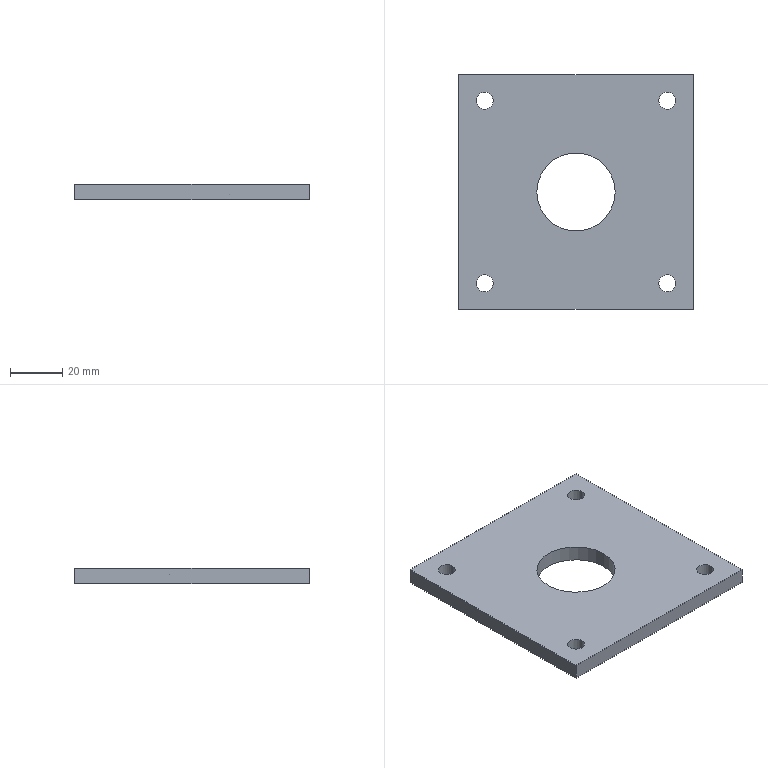Part | STEP file | Square tube fixing plate SGN-7-01 | 1 solid | 16 faces | box 90 x 90 x 6 mm | volume 43562 mm3 | cylinder 10 | plane 6 | commonest cylinder face diameters 6.5 x8 30 x2
STEP:
#1=CARTESIAN_POINT('',(0.,0.,0.));
#2=DIRECTION('',(0.,0.,1.));
#3=DIRECTION('',(1.,0.,0.));
#4=AXIS2_PLACEMENT_3D('',#1,#2,#3);
#5=CARTESIAN_POINT('',(38.25,35.,0.));
#6=VERTEX_POINT('',#5);
#7=CARTESIAN_POINT('',(38.25,35.,6.));
#8=VERTEX_POINT('',#7);
#9=CARTESIAN_POINT('',(38.25,35.,0.));
#10=DIRECTION('',(0.,0.,1.));
#11=VECTOR('',#10,1.);
#12=LINE('',#9,#11);
#13=CARTESIAN_POINT('',(35.,35.,0.));
#14=DIRECTION('',(0.,0.,1.));
#15=DIRECTION('',(1.,0.,0.));
#16=AXIS2_PLACEMENT_3D('',#13,#14,#15);
#17=CYLINDRICAL_SURFACE('',#16,3.25);
#18=CARTESIAN_POINT('',(6.283,0.));
#19=DIRECTION('',(0.,1.));
#20=VECTOR('',#19,1.);
#21=LINE('',#18,#20);
#22=(GEOMETRIC_REPRESENTATION_CONTEXT(2)PARAMETRIC_REPRESENTATION_CONTEXT()REPRESENTATION_CONTEXT('',''));
#23=DEFINITIONAL_REPRESENTATION('',(#21),#22);
#24=PCURVE('',#17,#23);
#25=CARTESIAN_POINT('',(35.,35.,0.));
#26=DIRECTION('',(0.,0.,1.));
#27=DIRECTION('',(1.,0.,0.));
#28=AXIS2_PLACEMENT_3D('',#25,#26,#27);
#29=CYLINDRICAL_SURFACE('',#28,3.25);
#30=CARTESIAN_POINT('',(0.,0.));
#31=DIRECTION('',(0.,1.));
#32=VECTOR('',#31,1.);
#33=LINE('',#30,#32);
#34=(GEOMETRIC_REPRESENTATION_CONTEXT(2)PARAMETRIC_REPRESENTATION_CONTEXT()REPRESENTATION_CONTEXT('',''));
#35=DEFINITIONAL_REPRESENTATION('',(#33),#34);
#36=PCURVE('',#29,#35);
#37=SURFACE_CURVE('',#12,(#24,#36),.PCURVE_S1.);
#38=EDGE_CURVE('',#6,#8,#37,.T.);
#39=ORIENTED_EDGE('',*,*,#38,.T.);
#40=CARTESIAN_POINT('',(31.75,35.,6.));
#41=VERTEX_POINT('',#40);
#42=CARTESIAN_POINT('',(35.,35.,6.));
#43=DIRECTION('',(0.,0.,1.));
#44=DIRECTION('',(1.,0.,0.));
#45=AXIS2_PLACEMENT_3D('',#42,#43,#44);
#46=CIRCLE('',#45,3.25);
#47=CARTESIAN_POINT('',(0.,6.));
#48=DIRECTION('',(1.,0.));
#49=VECTOR('',#48,1.);
#50=LINE('',#47,#49);
#51=(GEOMETRIC_REPRESENTATION_CONTEXT(2)PARAMETRIC_REPRESENTATION_CONTEXT()REPRESENTATION_CONTEXT('',''));
#52=DEFINITIONAL_REPRESENTATION('',(#50),#51);
#53=PCURVE('',#17,#52);
#54=CARTESIAN_POINT('',(0.,0.,6.));
#55=DIRECTION('',(0.,0.,-1.));
#56=DIRECTION('',(-1.,0.,0.));
#57=AXIS2_PLACEMENT_3D('',#54,#55,#56);
#58=PLANE('',#57);
#59=CARTESIAN_POINT('',(-38.25,35.));
#60=CARTESIAN_POINT('',(-38.25,40.629));
#61=CARTESIAN_POINT('',(-33.375,37.815));
#62=CARTESIAN_POINT('',(-28.5,35.));
#63=CARTESIAN_POINT('',(-33.375,32.185));
#64=CARTESIAN_POINT('',(-38.25,29.371));
#65=CARTESIAN_POINT('',(-38.25,35.));
#66=(BOUNDED_CURVE()B_SPLINE_CURVE(2,(#59,#60,#61,#62,#63,#64,#65),.UNSPECIFIED.,.T.,.F.)B_SPLINE_CURVE_WITH_KNOTS((1,2,2,2,2,1),(-2.094,0.,2.094,4.189,6.283,8.378),.UNSPECIFIED.)CURVE()GEOMETRIC_REPRESENTATION_ITEM()RATIONAL_B_SPLINE_CURVE((1.,0.5,1.,0.5,1.,0.5,1.))REPRESENTATION_ITEM(''));
#67=(GEOMETRIC_REPRESENTATION_CONTEXT(2)PARAMETRIC_REPRESENTATION_CONTEXT()REPRESENTATION_CONTEXT('',''));
#68=DEFINITIONAL_REPRESENTATION('',(#66),#67);
#69=PCURVE('',#58,#68);
#70=SURFACE_CURVE('',#46,(#53,#69),.PCURVE_S1.);
#71=EDGE_CURVE('',#41,#8,#70,.T.);
#72=ORIENTED_EDGE('',*,*,#71,.F.);
#73=CARTESIAN_POINT('',(31.75,35.,0.));
#74=VERTEX_POINT('',#73);
#75=CARTESIAN_POINT('',(31.75,35.,0.));
#76=DIRECTION('',(0.,0.,1.));
#77=VECTOR('',#76,1.);
#78=LINE('',#75,#77);
#79=CARTESIAN_POINT('',(3.142,0.));
#80=DIRECTION('',(0.,1.));
#81=VECTOR('',#80,1.);
#82=LINE('',#79,#81);
#83=(GEOMETRIC_REPRESENTATION_CONTEXT(2)PARAMETRIC_REPRESENTATION_CONTEXT()REPRESENTATION_CONTEXT('',''));
#84=DEFINITIONAL_REPRESENTATION('',(#82),#83);
#85=PCURVE('',#17,#84);
#86=CARTESIAN_POINT('',(3.142,0.));
#87=DIRECTION('',(0.,1.));
#88=VECTOR('',#87,1.);
#89=LINE('',#86,#88);
#90=(GEOMETRIC_REPRESENTATION_CONTEXT(2)PARAMETRIC_REPRESENTATION_CONTEXT()REPRESENTATION_CONTEXT('',''));
#91=DEFINITIONAL_REPRESENTATION('',(#89),#90);
#92=PCURVE('',#29,#91);
#93=SURFACE_CURVE('',#78,(#85,#92),.PCURVE_S1.);
#94=EDGE_CURVE('',#74,#41,#93,.T.);
#95=ORIENTED_EDGE('',*,*,#94,.F.);
#96=CARTESIAN_POINT('',(35.,35.,0.));
#97=DIRECTION('',(0.,0.,1.));
#98=DIRECTION('',(1.,0.,0.));
#99=AXIS2_PLACEMENT_3D('',#96,#97,#98);
#100=CIRCLE('',#99,3.25);
#101=CARTESIAN_POINT('',(0.,0.));
#102=DIRECTION('',(1.,0.));
#103=VECTOR('',#102,1.);
#104=LINE('',#101,#103);
#105=(GEOMETRIC_REPRESENTATION_CONTEXT(2)PARAMETRIC_REPRESENTATION_CONTEXT()REPRESENTATION_CONTEXT('',''));
#106=DEFINITIONAL_REPRESENTATION('',(#104),#105);
#107=PCURVE('',#17,#106);
#108=CARTESIAN_POINT('',(0.,0.,0.));
#109=DIRECTION('',(0.,0.,-1.));
#110=DIRECTION('',(-1.,0.,0.));
#111=AXIS2_PLACEMENT_3D('',#108,#109,#110);
#112=PLANE('',#111);
#113=CARTESIAN_POINT('',(-38.25,35.));
#114=CARTESIAN_POINT('',(-38.25,40.629));
#115=CARTESIAN_POINT('',(-33.375,37.815));
#116=CARTESIAN_POINT('',(-28.5,35.));
#117=CARTESIAN_POINT('',(-33.375,32.185));
#118=CARTESIAN_POINT('',(-38.25,29.371));
#119=CARTESIAN_POINT('',(-38.25,35.));
#120=(BOUNDED_CURVE()B_SPLINE_CURVE(2,(#113,#114,#115,#116,#117,#118,#119),.UNSPECIFIED.,.T.,.F.)B_SPLINE_CURVE_WITH_KNOTS((1,2,2,2,2,1),(-2.094,0.,2.094,4.189,6.283,8.378),.UNSPECIFIED.)CURVE()GEOMETRIC_REPRESENTATION_ITEM()RATIONAL_B_SPLINE_CURVE((1.,0.5,1.,0.5,1.,0.5,1.))REPRESENTATION_ITEM(''));
#121=(GEOMETRIC_REPRESENTATION_CONTEXT(2)PARAMETRIC_REPRESENTATION_CONTEXT()REPRESENTATION_CONTEXT('',''));
#122=DEFINITIONAL_REPRESENTATION('',(#120),#121);
#123=PCURVE('',#112,#122);
#124=SURFACE_CURVE('',#100,(#107,#123),.PCURVE_S1.);
#125=EDGE_CURVE('',#74,#6,#124,.T.);
#126=ORIENTED_EDGE('',*,*,#125,.T.);
#127=EDGE_LOOP('',(#39,#72,#95,#126));
#128=FACE_BOUND('',#127,.F.);
#129=ADVANCED_FACE('',(#128),#17,.F.);
#130=CARTESIAN_POINT('',(-31.75,-35.,0.));
#131=VERTEX_POINT('',#130);
#132=CARTESIAN_POINT('',(-31.75,-35.,6.));
#133=VERTEX_POINT('',#132);
#134=CARTESIAN_POINT('',(-31.75,-35.,0.));
#135=DIRECTION('',(0.,0.,1.));
#136=VECTOR('',#135,1.);
#137=LINE('',#134,#136);
#138=CARTESIAN_POINT('',(-35.,-35.,0.));
#139=DIRECTION('',(0.,0.,1.));
#140=DIRECTION('',(1.,0.,0.));
#141=AXIS2_PLACEMENT_3D('',#138,#139,#140);
#142=CYLINDRICAL_SURFACE('',#141,3.25);
#143=CARTESIAN_POINT('',(6.283,0.));
#144=DIRECTION('',(0.,1.));
#145=VECTOR('',#144,1.);
#146=LINE('',#143,#145);
#147=(GEOMETRIC_REPRESENTATION_CONTEXT(2)PARAMETRIC_REPRESENTATION_CONTEXT()REPRESENTATION_CONTEXT('',''));
#148=DEFINITIONAL_REPRESENTATION('',(#146),#147);
#149=PCURVE('',#142,#148);
#150=CARTESIAN_POINT('',(-35.,-35.,0.));
#151=DIRECTION('',(0.,0.,1.));
#152=DIRECTION('',(1.,0.,0.));
#153=AXIS2_PLACEMENT_3D('',#150,#151,#152);
#154=CYLINDRICAL_SURFACE('',#153,3.25);
#155=CARTESIAN_POINT('',(0.,0.));
#156=DIRECTION('',(0.,1.));
#157=VECTOR('',#156,1.);
#158=LINE('',#155,#157);
#159=(GEOMETRIC_REPRESENTATION_CONTEXT(2)PARAMETRIC_REPRESENTATION_CONTEXT()REPRESENTATION_CONTEXT('',''));
#160=DEFINITIONAL_REPRESENTATION('',(#158),#159);
#161=PCURVE('',#154,#160);
#162=SURFACE_CURVE('',#137,(#149,#161),.PCURVE_S1.);
#163=EDGE_CURVE('',#131,#133,#162,.T.);
#164=ORIENTED_EDGE('',*,*,#163,.T.);
#165=CARTESIAN_POINT('',(-38.25,-35.,6.));
#166=VERTEX_POINT('',#165);
#167=CARTESIAN_POINT('',(-35.,-35.,6.));
#168=DIRECTION('',(0.,0.,1.));
#169=DIRECTION('',(1.,0.,0.));
#170=AXIS2_PLACEMENT_3D('',#167,#168,#169);
#171=CIRCLE('',#170,3.25);
#172=CARTESIAN_POINT('',(0.,6.));
#173=DIRECTION('',(1.,0.));
#174=VECTOR('',#173,1.);
#175=LINE('',#172,#174);
#176=(GEOMETRIC_REPRESENTATION_CONTEXT(2)PARAMETRIC_REPRESENTATION_CONTEXT()REPRESENTATION_CONTEXT('',''));
#177=DEFINITIONAL_REPRESENTATION('',(#175),#176);
#178=PCURVE('',#142,#177);
#179=CARTESIAN_POINT('',(31.75,-35.));
#180=CARTESIAN_POINT('',(31.75,-29.371));
#181=CARTESIAN_POINT('',(36.625,-32.185));
#182=CARTESIAN_POINT('',(41.5,-35.));
#183=CARTESIAN_POINT('',(36.625,-37.815));
#184=CARTESIAN_POINT('',(31.75,-40.629));
#185=CARTESIAN_POINT('',(31.75,-35.));
#186=(BOUNDED_CURVE()B_SPLINE_CURVE(2,(#179,#180,#181,#182,#183,#184,#185),.UNSPECIFIED.,.T.,.F.)B_SPLINE_CURVE_WITH_KNOTS((1,2,2,2,2,1),(-2.094,0.,2.094,4.189,6.283,8.378),.UNSPECIFIED.)CURVE()GEOMETRIC_REPRESENTATION_ITEM()RATIONAL_B_SPLINE_CURVE((1.,0.5,1.,0.5,1.,0.5,1.))REPRESENTATION_ITEM(''));
#187=(GEOMETRIC_REPRESENTATION_CONTEXT(2)PARAMETRIC_REPRESENTATION_CONTEXT()REPRESENTATION_CONTEXT('',''));
#188=DEFINITIONAL_REPRESENTATION('',(#186),#187);
#189=PCURVE('',#58,#188);
#190=SURFACE_CURVE('',#171,(#178,#189),.PCURVE_S1.);
#191=EDGE_CURVE('',#166,#133,#190,.T.);
#192=ORIENTED_EDGE('',*,*,#191,.F.);
#193=CARTESIAN_POINT('',(-38.25,-35.,0.));
#194=VERTEX_POINT('',#193);
#195=CARTESIAN_POINT('',(-38.25,-35.,0.));
#196=DIRECTION('',(0.,0.,1.));
#197=VECTOR('',#196,1.);
#198=LINE('',#195,#197);
#199=CARTESIAN_POINT('',(3.142,0.));
#200=DIRECTION('',(0.,1.));
#201=VECTOR('',#200,1.);
#202=LINE('',#199,#201);
#203=(GEOMETRIC_REPRESENTATION_CONTEXT(2)PARAMETRIC_REPRESENTATION_CONTEXT()REPRESENTATION_CONTEXT('',''));
#204=DEFINITIONAL_REPRESENTATION('',(#202),#203);
#205=PCURVE('',#142,#204);
#206=CARTESIAN_POINT('',(3.142,0.));
#207=DIRECTION('',(0.,1.));
#208=VECTOR('',#207,1.);
#209=LINE('',#206,#208);
#210=(GEOMETRIC_REPRESENTATION_CONTEXT(2)PARAMETRIC_REPRESENTATION_CONTEXT()REPRESENTATION_CONTEXT('',''));
#211=DEFINITIONAL_REPRESENTATION('',(#209),#210);
#212=PCURVE('',#154,#211);
#213=SURFACE_CURVE('',#198,(#205,#212),.PCURVE_S1.);
#214=EDGE_CURVE('',#194,#166,#213,.T.);
#215=ORIENTED_EDGE('',*,*,#214,.F.);
#216=CARTESIAN_POINT('',(-35.,-35.,0.));
#217=DIRECTION('',(0.,0.,1.));
#218=DIRECTION('',(1.,0.,0.));
#219=AXIS2_PLACEMENT_3D('',#216,#217,#218);
#220=CIRCLE('',#219,3.25);
#221=CARTESIAN_POINT('',(0.,0.));
#222=DIRECTION('',(1.,0.));
#223=VECTOR('',#222,1.);
#224=LINE('',#221,#223);
#225=(GEOMETRIC_REPRESENTATION_CONTEXT(2)PARAMETRIC_REPRESENTATION_CONTEXT()REPRESENTATION_CONTEXT('',''));
#226=DEFINITIONAL_REPRESENTATION('',(#224),#225);
#227=PCURVE('',#142,#226);
#228=CARTESIAN_POINT('',(31.75,-35.));
#229=CARTESIAN_POINT('',(31.75,-29.371));
#230=CARTESIAN_POINT('',(36.625,-32.185));
#231=CARTESIAN_POINT('',(41.5,-35.));
#232=CARTESIAN_POINT('',(36.625,-37.815));
#233=CARTESIAN_POINT('',(31.75,-40.629));
#234=CARTESIAN_POINT('',(31.75,-35.));
#235=(BOUNDED_CURVE()B_SPLINE_CURVE(2,(#228,#229,#230,#231,#232,#233,#234),.UNSPECIFIED.,.T.,.F.)B_SPLINE_CURVE_WITH_KNOTS((1,2,2,2,2,1),(-2.094,0.,2.094,4.189,6.283,8.378),.UNSPECIFIED.)CURVE()GEOMETRIC_REPRESENTATION_ITEM()RATIONAL_B_SPLINE_CURVE((1.,0.5,1.,0.5,1.,0.5,1.))REPRESENTATION_ITEM(''));
#236=(GEOMETRIC_REPRESENTATION_CONTEXT(2)PARAMETRIC_REPRESENTATION_CONTEXT()REPRESENTATION_CONTEXT('',''));
#237=DEFINITIONAL_REPRESENTATION('',(#235),#236);
#238=PCURVE('',#112,#237);
#239=SURFACE_CURVE('',#220,(#227,#238),.PCURVE_S1.);
#240=EDGE_CURVE('',#194,#131,#239,.T.);
#241=ORIENTED_EDGE('',*,*,#240,.T.);
#242=EDGE_LOOP('',(#164,#192,#215,#241));
#243=FACE_BOUND('',#242,.F.);
#244=ADVANCED_FACE('',(#243),#142,.F.);
#245=CARTESIAN_POINT('',(38.25,-35.,0.));
#246=VERTEX_POINT('',#245);
#247=CARTESIAN_POINT('',(38.25,-35.,6.));
#248=VERTEX_POINT('',#247);
#249=CARTESIAN_POINT('',(38.25,-35.,0.));
#250=DIRECTION('',(0.,0.,1.));
#251=VECTOR('',#250,1.);
#252=LINE('',#249,#251);
#253=CARTESIAN_POINT('',(35.,-35.,0.));
#254=DIRECTION('',(0.,0.,1.));
#255=DIRECTION('',(1.,0.,0.));
#256=AXIS2_PLACEMENT_3D('',#253,#254,#255);
#257=CYLINDRICAL_SURFACE('',#256,3.25);
#258=CARTESIAN_POINT('',(6.283,0.));
#259=DIRECTION('',(0.,1.));
#260=VECTOR('',#259,1.);
#261=LINE('',#258,#260);
#262=(GEOMETRIC_REPRESENTATION_CONTEXT(2)PARAMETRIC_REPRESENTATION_CONTEXT()REPRESENTATION_CONTEXT('',''));
#263=DEFINITIONAL_REPRESENTATION('',(#261),#262);
#264=PCURVE('',#257,#263);
#265=CARTESIAN_POINT('',(35.,-35.,0.));
#266=DIRECTION('',(0.,0.,1.));
#267=DIRECTION('',(1.,0.,0.));
#268=AXIS2_PLACEMENT_3D('',#265,#266,#267);
#269=CYLINDRICAL_SURFACE('',#268,3.25);
#270=CARTESIAN_POINT('',(0.,0.));
#271=DIRECTION('',(0.,1.));
#272=VECTOR('',#271,1.);
#273=LINE('',#270,#272);
#274=(GEOMETRIC_REPRESENTATION_CONTEXT(2)PARAMETRIC_REPRESENTATION_CONTEXT()REPRESENTATION_CONTEXT('',''));
#275=DEFINITIONAL_REPRESENTATION('',(#273),#274);
#276=PCURVE('',#269,#275);
#277=SURFACE_CURVE('',#252,(#264,#276),.PCURVE_S1.);
#278=EDGE_CURVE('',#246,#248,#277,.T.);
#279=ORIENTED_EDGE('',*,*,#278,.T.);
#280=CARTESIAN_POINT('',(31.75,-35.,6.));
#281=VERTEX_POINT('',#280);
#282=CARTESIAN_POINT('',(35.,-35.,6.));
#283=DIRECTION('',(0.,0.,1.));
#284=DIRECTION('',(1.,0.,0.));
#285=AXIS2_PLACEMENT_3D('',#282,#283,#284);
#286=CIRCLE('',#285,3.25);
#287=CARTESIAN_POINT('',(0.,6.));
#288=DIRECTION('',(1.,0.));
#289=VECTOR('',#288,1.);
#290=LINE('',#287,#289);
#291=(GEOMETRIC_REPRESENTATION_CONTEXT(2)PARAMETRIC_REPRESENTATION_CONTEXT()REPRESENTATION_CONTEXT('',''));
#292=DEFINITIONAL_REPRESENTATION('',(#290),#291);
#293=PCURVE('',#257,#292);
#294=CARTESIAN_POINT('',(-38.25,-35.));
#295=CARTESIAN_POINT('',(-38.25,-29.371));
#296=CARTESIAN_POINT('',(-33.375,-32.185));
#297=CARTESIAN_POINT('',(-28.5,-35.));
#298=CARTESIAN_POINT('',(-33.375,-37.815));
#299=CARTESIAN_POINT('',(-38.25,-40.629));
#300=CARTESIAN_POINT('',(-38.25,-35.));
#301=(BOUNDED_CURVE()B_SPLINE_CURVE(2,(#294,#295,#296,#297,#298,#299,#300),.UNSPECIFIED.,.T.,.F.)B_SPLINE_CURVE_WITH_KNOTS((1,2,2,2,2,1),(-2.094,0.,2.094,4.189,6.283,8.378),.UNSPECIFIED.)CURVE()GEOMETRIC_REPRESENTATION_ITEM()RATIONAL_B_SPLINE_CURVE((1.,0.5,1.,0.5,1.,0.5,1.))REPRESENTATION_ITEM(''));
#302=(GEOMETRIC_REPRESENTATION_CONTEXT(2)PARAMETRIC_REPRESENTATION_CONTEXT()REPRESENTATION_CONTEXT('',''));
#303=DEFINITIONAL_REPRESENTATION('',(#301),#302);
#304=PCURVE('',#58,#303);
#305=SURFACE_CURVE('',#286,(#293,#304),.PCURVE_S1.);
#306=EDGE_CURVE('',#281,#248,#305,.T.);
#307=ORIENTED_EDGE('',*,*,#306,.F.);
#308=CARTESIAN_POINT('',(31.75,-35.,0.));
#309=VERTEX_POINT('',#308);
#310=CARTESIAN_POINT('',(31.75,-35.,0.));
#311=DIRECTION('',(0.,0.,1.));
#312=VECTOR('',#311,1.);
#313=LINE('',#310,#312);
#314=CARTESIAN_POINT('',(3.142,0.));
#315=DIRECTION('',(0.,1.));
#316=VECTOR('',#315,1.);
#317=LINE('',#314,#316);
#318=(GEOMETRIC_REPRESENTATION_CONTEXT(2)PARAMETRIC_REPRESENTATION_CONTEXT()REPRESENTATION_CONTEXT('',''));
#319=DEFINITIONAL_REPRESENTATION('',(#317),#318);
#320=PCURVE('',#257,#319);
#321=CARTESIAN_POINT('',(3.142,0.));
#322=DIRECTION('',(0.,1.));
#323=VECTOR('',#322,1.);
#324=LINE('',#321,#323);
#325=(GEOMETRIC_REPRESENTATION_CONTEXT(2)PARAMETRIC_REPRESENTATION_CONTEXT()REPRESENTATION_CONTEXT('',''));
#326=DEFINITIONAL_REPRESENTATION('',(#324),#325);
#327=PCURVE('',#269,#326);
#328=SURFACE_CURVE('',#313,(#320,#327),.PCURVE_S1.);
#329=EDGE_CURVE('',#309,#281,#328,.T.);
#330=ORIENTED_EDGE('',*,*,#329,.F.);
#331=CARTESIAN_POINT('',(35.,-35.,0.));
#332=DIRECTION('',(0.,0.,1.));
#333=DIRECTION('',(1.,0.,0.));
#334=AXIS2_PLACEMENT_3D('',#331,#332,#333);
#335=CIRCLE('',#334,3.25);
#336=CARTESIAN_POINT('',(0.,0.));
#337=DIRECTION('',(1.,0.));
#338=VECTOR('',#337,1.);
#339=LINE('',#336,#338);
#340=(GEOMETRIC_REPRESENTATION_CONTEXT(2)PARAMETRIC_REPRESENTATION_CONTEXT()REPRESENTATION_CONTEXT('',''));
#341=DEFINITIONAL_REPRESENTATION('',(#339),#340);
#342=PCURVE('',#257,#341);
#343=CARTESIAN_POINT('',(-38.25,-35.));
#344=CARTESIAN_POINT('',(-38.25,-29.371));
#345=CARTESIAN_POINT('',(-33.375,-32.185));
#346=CARTESIAN_POINT('',(-28.5,-35.));
#347=CARTESIAN_POINT('',(-33.375,-37.815));
#348=CARTESIAN_POINT('',(-38.25,-40.629));
#349=CARTESIAN_POINT('',(-38.25,-35.));
#350=(BOUNDED_CURVE()B_SPLINE_CURVE(2,(#343,#344,#345,#346,#347,#348,#349),.UNSPECIFIED.,.T.,.F.)B_SPLINE_CURVE_WITH_KNOTS((1,2,2,2,2,1),(-2.094,0.,2.094,4.189,6.283,8.378),.UNSPECIFIED.)CURVE()GEOMETRIC_REPRESENTATION_ITEM()RATIONAL_B_SPLINE_CURVE((1.,0.5,1.,0.5,1.,0.5,1.))REPRESENTATION_ITEM(''));
#351=(GEOMETRIC_REPRESENTATION_CONTEXT(2)PARAMETRIC_REPRESENTATION_CONTEXT()REPRESENTATION_CONTEXT('',''));
#352=DEFINITIONAL_REPRESENTATION('',(#350),#351);
#353=PCURVE('',#112,#352);
#354=SURFACE_CURVE('',#335,(#342,#353),.PCURVE_S1.);
#355=EDGE_CURVE('',#309,#246,#354,.T.);
#356=ORIENTED_EDGE('',*,*,#355,.T.);
#357=EDGE_LOOP('',(#279,#307,#330,#356));
#358=FACE_BOUND('',#357,.F.);
#359=ADVANCED_FACE('',(#358),#257,.F.);
#360=CARTESIAN_POINT('',(15.,0.,0.));
#361=VERTEX_POINT('',#360);
#362=CARTESIAN_POINT('',(15.,0.,6.));
#363=VERTEX_POINT('',#362);
#364=CARTESIAN_POINT('',(15.,0.,0.));
#365=DIRECTION('',(0.,0.,1.));
#366=VECTOR('',#365,1.);
#367=LINE('',#364,#366);
#368=CARTESIAN_POINT('',(0.,0.,0.));
#369=DIRECTION('',(0.,0.,1.));
#370=DIRECTION('',(1.,0.,0.));
#371=AXIS2_PLACEMENT_3D('',#368,#369,#370);
#372=CYLINDRICAL_SURFACE('',#371,15.);
#373=CARTESIAN_POINT('',(6.283,0.));
#374=DIRECTION('',(0.,1.));
#375=VECTOR('',#374,1.);
#376=LINE('',#373,#375);
#377=(GEOMETRIC_REPRESENTATION_CONTEXT(2)PARAMETRIC_REPRESENTATION_CONTEXT()REPRESENTATION_CONTEXT('',''));
#378=DEFINITIONAL_REPRESENTATION('',(#376),#377);
#379=PCURVE('',#372,#378);
#380=CARTESIAN_POINT('',(0.,0.,0.));
#381=DIRECTION('',(0.,0.,1.));
#382=DIRECTION('',(1.,0.,0.));
#383=AXIS2_PLACEMENT_3D('',#380,#381,#382);
#384=CYLINDRICAL_SURFACE('',#383,15.);
#385=CARTESIAN_POINT('',(0.,0.));
#386=DIRECTION('',(0.,1.));
#387=VECTOR('',#386,1.);
#388=LINE('',#385,#387);
#389=(GEOMETRIC_REPRESENTATION_CONTEXT(2)PARAMETRIC_REPRESENTATION_CONTEXT()REPRESENTATION_CONTEXT('',''));
#390=DEFINITIONAL_REPRESENTATION('',(#388),#389);
#391=PCURVE('',#384,#390);
#392=SURFACE_CURVE('',#367,(#379,#391),.PCURVE_S1.);
#393=EDGE_CURVE('',#361,#363,#392,.T.);
#394=ORIENTED_EDGE('',*,*,#393,.T.);
#395=CARTESIAN_POINT('',(-15.,0.,6.));
#396=VERTEX_POINT('',#395);
#397=CARTESIAN_POINT('',(0.,0.,6.));
#398=DIRECTION('',(0.,0.,1.));
#399=DIRECTION('',(1.,0.,0.));
#400=AXIS2_PLACEMENT_3D('',#397,#398,#399);
#401=CIRCLE('',#400,15.);
#402=CARTESIAN_POINT('',(0.,6.));
#403=DIRECTION('',(1.,0.));
#404=VECTOR('',#403,1.);
#405=LINE('',#402,#404);
#406=(GEOMETRIC_REPRESENTATION_CONTEXT(2)PARAMETRIC_REPRESENTATION_CONTEXT()REPRESENTATION_CONTEXT('',''));
#407=DEFINITIONAL_REPRESENTATION('',(#405),#406);
#408=PCURVE('',#372,#407);
#409=CARTESIAN_POINT('',(-15.,0.));
#410=CARTESIAN_POINT('',(-15.,25.981));
#411=CARTESIAN_POINT('',(7.5,12.99));
#412=CARTESIAN_POINT('',(30.,0.));
#413=CARTESIAN_POINT('',(7.5,-12.99));
#414=CARTESIAN_POINT('',(-15.,-25.981));
#415=CARTESIAN_POINT('',(-15.,0.));
#416=(BOUNDED_CURVE()B_SPLINE_CURVE(2,(#409,#410,#411,#412,#413,#414,#415),.UNSPECIFIED.,.T.,.F.)B_SPLINE_CURVE_WITH_KNOTS((1,2,2,2,2,1),(-2.094,0.,2.094,4.189,6.283,8.378),.UNSPECIFIED.)CURVE()GEOMETRIC_REPRESENTATION_ITEM()RATIONAL_B_SPLINE_CURVE((1.,0.5,1.,0.5,1.,0.5,1.))REPRESENTATION_ITEM(''));
#417=(GEOMETRIC_REPRESENTATION_CONTEXT(2)PARAMETRIC_REPRESENTATION_CONTEXT()REPRESENTATION_CONTEXT('',''));
#418=DEFINITIONAL_REPRESENTATION('',(#416),#417);
#419=PCURVE('',#58,#418);
#420=SURFACE_CURVE('',#401,(#408,#419),.PCURVE_S1.);
#421=EDGE_CURVE('',#396,#363,#420,.T.);
#422=ORIENTED_EDGE('',*,*,#421,.F.);
#423=CARTESIAN_POINT('',(-15.,0.,0.));
#424=VERTEX_POINT('',#423);
#425=CARTESIAN_POINT('',(-15.,0.,0.));
#426=DIRECTION('',(0.,0.,1.));
#427=VECTOR('',#426,1.);
#428=LINE('',#425,#427);
#429=CARTESIAN_POINT('',(3.142,0.));
#430=DIRECTION('',(0.,1.));
#431=VECTOR('',#430,1.);
#432=LINE('',#429,#431);
#433=(GEOMETRIC_REPRESENTATION_CONTEXT(2)PARAMETRIC_REPRESENTATION_CONTEXT()REPRESENTATION_CONTEXT('',''));
#434=DEFINITIONAL_REPRESENTATION('',(#432),#433);
#435=PCURVE('',#372,#434);
#436=CARTESIAN_POINT('',(3.142,0.));
#437=DIRECTION('',(0.,1.));
#438=VECTOR('',#437,1.);
#439=LINE('',#436,#438);
#440=(GEOMETRIC_REPRESENTATION_CONTEXT(2)PARAMETRIC_REPRESENTATION_CONTEXT()REPRESENTATION_CONTEXT('',''));
#441=DEFINITIONAL_REPRESENTATION('',(#439),#440);
#442=PCURVE('',#384,#441);
#443=SURFACE_CURVE('',#428,(#435,#442),.PCURVE_S1.);
#444=EDGE_CURVE('',#424,#396,#443,.T.);
#445=ORIENTED_EDGE('',*,*,#444,.F.);
#446=CARTESIAN_POINT('',(0.,0.,0.));
#447=DIRECTION('',(0.,0.,1.));
#448=DIRECTION('',(1.,0.,0.));
#449=AXIS2_PLACEMENT_3D('',#446,#447,#448);
#450=CIRCLE('',#449,15.);
#451=CARTESIAN_POINT('',(0.,0.));
#452=DIRECTION('',(1.,0.));
#453=VECTOR('',#452,1.);
#454=LINE('',#451,#453);
#455=(GEOMETRIC_REPRESENTATION_CONTEXT(2)PARAMETRIC_REPRESENTATION_CONTEXT()REPRESENTATION_CONTEXT('',''));
#456=DEFINITIONAL_REPRESENTATION('',(#454),#455);
#457=PCURVE('',#372,#456);
#458=CARTESIAN_POINT('',(-15.,0.));
#459=CARTESIAN_POINT('',(-15.,25.981));
#460=CARTESIAN_POINT('',(7.5,12.99));
#461=CARTESIAN_POINT('',(30.,0.));
#462=CARTESIAN_POINT('',(7.5,-12.99));
#463=CARTESIAN_POINT('',(-15.,-25.981));
#464=CARTESIAN_POINT('',(-15.,0.));
#465=(BOUNDED_CURVE()B_SPLINE_CURVE(2,(#458,#459,#460,#461,#462,#463,#464),.UNSPECIFIED.,.T.,.F.)B_SPLINE_CURVE_WITH_KNOTS((1,2,2,2,2,1),(-2.094,0.,2.094,4.189,6.283,8.378),.UNSPECIFIED.)CURVE()GEOMETRIC_REPRESENTATION_ITEM()RATIONAL_B_SPLINE_CURVE((1.,0.5,1.,0.5,1.,0.5,1.))REPRESENTATION_ITEM(''));
#466=(GEOMETRIC_REPRESENTATION_CONTEXT(2)PARAMETRIC_REPRESENTATION_CONTEXT()REPRESENTATION_CONTEXT('',''));
#467=DEFINITIONAL_REPRESENTATION('',(#465),#466);
#468=PCURVE('',#112,#467);
#469=SURFACE_CURVE('',#450,(#457,#468),.PCURVE_S1.);
#470=EDGE_CURVE('',#424,#361,#469,.T.);
#471=ORIENTED_EDGE('',*,*,#470,.T.);
#472=EDGE_LOOP('',(#394,#422,#445,#471));
#473=FACE_BOUND('',#472,.F.);
#474=ADVANCED_FACE('',(#473),#372,.F.);
#475=CARTESIAN_POINT('',(-31.75,35.,0.));
#476=VERTEX_POINT('',#475);
#477=CARTESIAN_POINT('',(-31.75,35.,6.));
#478=VERTEX_POINT('',#477);
#479=CARTESIAN_POINT('',(-31.75,35.,0.));
#480=DIRECTION('',(0.,0.,1.));
#481=VECTOR('',#480,1.);
#482=LINE('',#479,#481);
#483=CARTESIAN_POINT('',(-35.,35.,0.));
#484=DIRECTION('',(0.,0.,1.));
#485=DIRECTION('',(1.,0.,0.));
#486=AXIS2_PLACEMENT_3D('',#483,#484,#485);
#487=CYLINDRICAL_SURFACE('',#486,3.25);
#488=CARTESIAN_POINT('',(6.283,0.));
#489=DIRECTION('',(0.,1.));
#490=VECTOR('',#489,1.);
#491=LINE('',#488,#490);
#492=(GEOMETRIC_REPRESENTATION_CONTEXT(2)PARAMETRIC_REPRESENTATION_CONTEXT()REPRESENTATION_CONTEXT('',''));
#493=DEFINITIONAL_REPRESENTATION('',(#491),#492);
#494=PCURVE('',#487,#493);
#495=CARTESIAN_POINT('',(-35.,35.,0.));
#496=DIRECTION('',(0.,0.,1.));
#497=DIRECTION('',(1.,0.,0.));
#498=AXIS2_PLACEMENT_3D('',#495,#496,#497);
#499=CYLINDRICAL_SURFACE('',#498,3.25);
#500=CARTESIAN_POINT('',(0.,0.));
#501=DIRECTION('',(0.,1.));
#502=VECTOR('',#501,1.);
#503=LINE('',#500,#502);
#504=(GEOMETRIC_REPRESENTATION_CONTEXT(2)PARAMETRIC_REPRESENTATION_CONTEXT()REPRESENTATION_CONTEXT('',''));
#505=DEFINITIONAL_REPRESENTATION('',(#503),#504);
#506=PCURVE('',#499,#505);
#507=SURFACE_CURVE('',#482,(#494,#506),.PCURVE_S1.);
#508=EDGE_CURVE('',#476,#478,#507,.T.);
#509=ORIENTED_EDGE('',*,*,#508,.T.);
#510=CARTESIAN_POINT('',(-38.25,35.,6.));
#511=VERTEX_POINT('',#510);
#512=CARTESIAN_POINT('',(-35.,35.,6.));
#513=DIRECTION('',(0.,0.,1.));
#514=DIRECTION('',(1.,0.,0.));
#515=AXIS2_PLACEMENT_3D('',#512,#513,#514);
#516=CIRCLE('',#515,3.25);
#517=CARTESIAN_POINT('',(0.,6.));
#518=DIRECTION('',(1.,0.));
#519=VECTOR('',#518,1.);
#520=LINE('',#517,#519);
#521=(GEOMETRIC_REPRESENTATION_CONTEXT(2)PARAMETRIC_REPRESENTATION_CONTEXT()REPRESENTATION_CONTEXT('',''));
#522=DEFINITIONAL_REPRESENTATION('',(#520),#521);
#523=PCURVE('',#487,#522);
#524=CARTESIAN_POINT('',(31.75,35.));
#525=CARTESIAN_POINT('',(31.75,40.629));
#526=CARTESIAN_POINT('',(36.625,37.815));
#527=CARTESIAN_POINT('',(41.5,35.));
#528=CARTESIAN_POINT('',(36.625,32.185));
#529=CARTESIAN_POINT('',(31.75,29.371));
#530=CARTESIAN_POINT('',(31.75,35.));
#531=(BOUNDED_CURVE()B_SPLINE_CURVE(2,(#524,#525,#526,#527,#528,#529,#530),.UNSPECIFIED.,.T.,.F.)B_SPLINE_CURVE_WITH_KNOTS((1,2,2,2,2,1),(-2.094,0.,2.094,4.189,6.283,8.378),.UNSPECIFIED.)CURVE()GEOMETRIC_REPRESENTATION_ITEM()RATIONAL_B_SPLINE_CURVE((1.,0.5,1.,0.5,1.,0.5,1.))REPRESENTATION_ITEM(''));
#532=(GEOMETRIC_REPRESENTATION_CONTEXT(2)PARAMETRIC_REPRESENTATION_CONTEXT()REPRESENTATION_CONTEXT('',''));
#533=DEFINITIONAL_REPRESENTATION('',(#531),#532);
#534=PCURVE('',#58,#533);
#535=SURFACE_CURVE('',#516,(#523,#534),.PCURVE_S1.);
#536=EDGE_CURVE('',#511,#478,#535,.T.);
#537=ORIENTED_EDGE('',*,*,#536,.F.);
#538=CARTESIAN_POINT('',(-38.25,35.,0.));
#539=VERTEX_POINT('',#538);
#540=CARTESIAN_POINT('',(-38.25,35.,0.));
#541=DIRECTION('',(0.,0.,1.));
#542=VECTOR('',#541,1.);
#543=LINE('',#540,#542);
#544=CARTESIAN_POINT('',(3.142,0.));
#545=DIRECTION('',(0.,1.));
#546=VECTOR('',#545,1.);
#547=LINE('',#544,#546);
#548=(GEOMETRIC_REPRESENTATION_CONTEXT(2)PARAMETRIC_REPRESENTATION_CONTEXT()REPRESENTATION_CONTEXT('',''));
#549=DEFINITIONAL_REPRESENTATION('',(#547),#548);
#550=PCURVE('',#487,#549);
#551=CARTESIAN_POINT('',(3.142,0.));
#552=DIRECTION('',(0.,1.));
#553=VECTOR('',#552,1.);
#554=LINE('',#551,#553);
#555=(GEOMETRIC_REPRESENTATION_CONTEXT(2)PARAMETRIC_REPRESENTATION_CONTEXT()REPRESENTATION_CONTEXT('',''));
#556=DEFINITIONAL_REPRESENTATION('',(#554),#555);
#557=PCURVE('',#499,#556);
#558=SURFACE_CURVE('',#543,(#550,#557),.PCURVE_S1.);
#559=EDGE_CURVE('',#539,#511,#558,.T.);
#560=ORIENTED_EDGE('',*,*,#559,.F.);
#561=CARTESIAN_POINT('',(-35.,35.,0.));
#562=DIRECTION('',(0.,0.,1.));
#563=DIRECTION('',(1.,0.,0.));
#564=AXIS2_PLACEMENT_3D('',#561,#562,#563);
#565=CIRCLE('',#564,3.25);
#566=CARTESIAN_POINT('',(0.,0.));
#567=DIRECTION('',(1.,0.));
#568=VECTOR('',#567,1.);
#569=LINE('',#566,#568);
#570=(GEOMETRIC_REPRESENTATION_CONTEXT(2)PARAMETRIC_REPRESENTATION_CONTEXT()REPRESENTATION_CONTEXT('',''));
#571=DEFINITIONAL_REPRESENTATION('',(#569),#570);
#572=PCURVE('',#487,#571);
#573=CARTESIAN_POINT('',(31.75,35.));
#574=CARTESIAN_POINT('',(31.75,40.629));
#575=CARTESIAN_POINT('',(36.625,37.815));
#576=CARTESIAN_POINT('',(41.5,35.));
#577=CARTESIAN_POINT('',(36.625,32.185));
#578=CARTESIAN_POINT('',(31.75,29.371));
#579=CARTESIAN_POINT('',(31.75,35.));
#580=(BOUNDED_CURVE()B_SPLINE_CURVE(2,(#573,#574,#575,#576,#577,#578,#579),.UNSPECIFIED.,.T.,.F.)B_SPLINE_CURVE_WITH_KNOTS((1,2,2,2,2,1),(-2.094,0.,2.094,4.189,6.283,8.378),.UNSPECIFIED.)CURVE()GEOMETRIC_REPRESENTATION_ITEM()RATIONAL_B_SPLINE_CURVE((1.,0.5,1.,0.5,1.,0.5,1.))REPRESENTATION_ITEM(''));
#581=(GEOMETRIC_REPRESENTATION_CONTEXT(2)PARAMETRIC_REPRESENTATION_CONTEXT()REPRESENTATION_CONTEXT('',''));
#582=DEFINITIONAL_REPRESENTATION('',(#580),#581);
#583=PCURVE('',#112,#582);
#584=SURFACE_CURVE('',#565,(#572,#583),.PCURVE_S1.);
#585=EDGE_CURVE('',#539,#476,#584,.T.);
#586=ORIENTED_EDGE('',*,*,#585,.T.);
#587=EDGE_LOOP('',(#509,#537,#560,#586));
#588=FACE_BOUND('',#587,.F.);
#589=ADVANCED_FACE('',(#588),#487,.F.);
#590=CARTESIAN_POINT('',(45.,-45.,0.));
#591=VERTEX_POINT('',#590);
#592=CARTESIAN_POINT('',(45.,45.,0.));
#593=VERTEX_POINT('',#592);
#594=CARTESIAN_POINT('',(45.,-45.,0.));
#595=DIRECTION('',(0.,1.,0.));
#596=VECTOR('',#595,1.);
#597=LINE('',#594,#596);
#598=CARTESIAN_POINT('',(45.,-45.,6.));
#599=DIRECTION('',(-1.,0.,0.));
#600=DIRECTION('',(0.,0.,1.));
#601=AXIS2_PLACEMENT_3D('',#598,#599,#600);
#602=PLANE('',#601);
#603=CARTESIAN_POINT('',(-6.,0.));
#604=DIRECTION('',(0.,1.));
#605=VECTOR('',#604,1.);
#606=LINE('',#603,#605);
#607=(GEOMETRIC_REPRESENTATION_CONTEXT(2)PARAMETRIC_REPRESENTATION_CONTEXT()REPRESENTATION_CONTEXT('',''));
#608=DEFINITIONAL_REPRESENTATION('',(#606),#607);
#609=PCURVE('',#602,#608);
#610=CARTESIAN_POINT('',(-45.,-45.));
#611=DIRECTION('',(0.,1.));
#612=VECTOR('',#611,1.);
#613=LINE('',#610,#612);
#614=(GEOMETRIC_REPRESENTATION_CONTEXT(2)PARAMETRIC_REPRESENTATION_CONTEXT()REPRESENTATION_CONTEXT('',''));
#615=DEFINITIONAL_REPRESENTATION('',(#613),#614);
#616=PCURVE('',#112,#615);
#617=SURFACE_CURVE('',#597,(#609,#616),.PCURVE_S1.);
#618=EDGE_CURVE('',#591,#593,#617,.T.);
#619=ORIENTED_EDGE('',*,*,#618,.T.);
#620=CARTESIAN_POINT('',(45.,45.,6.));
#621=VERTEX_POINT('',#620);
#622=CARTESIAN_POINT('',(45.,45.,6.));
#623=DIRECTION('',(0.,0.,-1.));
#624=VECTOR('',#623,1.);
#625=LINE('',#622,#624);
#626=CARTESIAN_POINT('',(0.,90.));
#627=DIRECTION('',(-1.,0.));
#628=VECTOR('',#627,1.);
#629=LINE('',#626,#628);
#630=(GEOMETRIC_REPRESENTATION_CONTEXT(2)PARAMETRIC_REPRESENTATION_CONTEXT()REPRESENTATION_CONTEXT('',''));
#631=DEFINITIONAL_REPRESENTATION('',(#629),#630);
#632=PCURVE('',#602,#631);
#633=CARTESIAN_POINT('',(-45.,45.,6.));
#634=DIRECTION('',(0.,-1.,0.));
#635=DIRECTION('',(0.,0.,-1.));
#636=AXIS2_PLACEMENT_3D('',#633,#634,#635);
#637=PLANE('',#636);
#638=CARTESIAN_POINT('',(0.,90.));
#639=DIRECTION('',(1.,0.));
#640=VECTOR('',#639,1.);
#641=LINE('',#638,#640);
#642=(GEOMETRIC_REPRESENTATION_CONTEXT(2)PARAMETRIC_REPRESENTATION_CONTEXT()REPRESENTATION_CONTEXT('',''));
#643=DEFINITIONAL_REPRESENTATION('',(#641),#642);
#644=PCURVE('',#637,#643);
#645=SURFACE_CURVE('',#625,(#632,#644),.PCURVE_S1.);
#646=EDGE_CURVE('',#621,#593,#645,.T.);
#647=ORIENTED_EDGE('',*,*,#646,.F.);
#648=CARTESIAN_POINT('',(45.,-45.,6.));
#649=VERTEX_POINT('',#648);
#650=CARTESIAN_POINT('',(45.,-45.,6.));
#651=DIRECTION('',(0.,1.,0.));
#652=VECTOR('',#651,1.);
#653=LINE('',#650,#652);
#654=CARTESIAN_POINT('',(0.,0.));
#655=DIRECTION('',(0.,1.));
#656=VECTOR('',#655,1.);
#657=LINE('',#654,#656);
#658=(GEOMETRIC_REPRESENTATION_CONTEXT(2)PARAMETRIC_REPRESENTATION_CONTEXT()REPRESENTATION_CONTEXT('',''));
#659=DEFINITIONAL_REPRESENTATION('',(#657),#658);
#660=PCURVE('',#602,#659);
#661=CARTESIAN_POINT('',(-45.,-45.));
#662=DIRECTION('',(0.,1.));
#663=VECTOR('',#662,1.);
#664=LINE('',#661,#663);
#665=(GEOMETRIC_REPRESENTATION_CONTEXT(2)PARAMETRIC_REPRESENTATION_CONTEXT()REPRESENTATION_CONTEXT('',''));
#666=DEFINITIONAL_REPRESENTATION('',(#664),#665);
#667=PCURVE('',#58,#666);
#668=SURFACE_CURVE('',#653,(#660,#667),.PCURVE_S1.);
#669=EDGE_CURVE('',#649,#621,#668,.T.);
#670=ORIENTED_EDGE('',*,*,#669,.F.);
#671=CARTESIAN_POINT('',(45.,-45.,6.));
#672=DIRECTION('',(0.,0.,-1.));
#673=VECTOR('',#672,1.);
#674=LINE('',#671,#673);
#675=CARTESIAN_POINT('',(0.,0.));
#676=DIRECTION('',(-1.,0.));
#677=VECTOR('',#676,1.);
#678=LINE('',#675,#677);
#679=(GEOMETRIC_REPRESENTATION_CONTEXT(2)PARAMETRIC_REPRESENTATION_CONTEXT()REPRESENTATION_CONTEXT('',''));
#680=DEFINITIONAL_REPRESENTATION('',(#678),#679);
#681=PCURVE('',#602,#680);
#682=CARTESIAN_POINT('',(-45.,-45.,6.));
#683=DIRECTION('',(0.,1.,0.));
#684=DIRECTION('',(0.,0.,1.));
#685=AXIS2_PLACEMENT_3D('',#682,#683,#684);
#686=PLANE('',#685);
#687=CARTESIAN_POINT('',(0.,90.));
#688=DIRECTION('',(-1.,0.));
#689=VECTOR('',#688,1.);
#690=LINE('',#687,#689);
#691=(GEOMETRIC_REPRESENTATION_CONTEXT(2)PARAMETRIC_REPRESENTATION_CONTEXT()REPRESENTATION_CONTEXT('',''));
#692=DEFINITIONAL_REPRESENTATION('',(#690),#691);
#693=PCURVE('',#686,#692);
#694=SURFACE_CURVE('',#674,(#681,#693),.PCURVE_S1.);
#695=EDGE_CURVE('',#649,#591,#694,.T.);
#696=ORIENTED_EDGE('',*,*,#695,.T.);
#697=EDGE_LOOP('',(#619,#647,#670,#696));
#698=FACE_BOUND('',#697,.T.);
#699=ADVANCED_FACE('',(#698),#602,.F.);
#700=CARTESIAN_POINT('',(-45.,45.,0.));
#701=VERTEX_POINT('',#700);
#702=CARTESIAN_POINT('',(-45.,45.,0.));
#703=DIRECTION('',(-1.,0.,0.));
#704=VECTOR('',#703,1.);
#705=LINE('',#702,#704);
#706=CARTESIAN_POINT('',(6.,0.));
#707=DIRECTION('',(0.,-1.));
#708=VECTOR('',#707,1.);
#709=LINE('',#706,#708);
#710=(GEOMETRIC_REPRESENTATION_CONTEXT(2)PARAMETRIC_REPRESENTATION_CONTEXT()REPRESENTATION_CONTEXT('',''));
#711=DEFINITIONAL_REPRESENTATION('',(#709),#710);
#712=PCURVE('',#637,#711);
#713=CARTESIAN_POINT('',(45.,45.));
#714=DIRECTION('',(1.,0.));
#715=VECTOR('',#714,1.);
#716=LINE('',#713,#715);
#717=(GEOMETRIC_REPRESENTATION_CONTEXT(2)PARAMETRIC_REPRESENTATION_CONTEXT()REPRESENTATION_CONTEXT('',''));
#718=DEFINITIONAL_REPRESENTATION('',(#716),#717);
#719=PCURVE('',#112,#718);
#720=SURFACE_CURVE('',#705,(#712,#719),.PCURVE_S1.);
#721=EDGE_CURVE('',#593,#701,#720,.T.);
#722=ORIENTED_EDGE('',*,*,#721,.T.);
#723=CARTESIAN_POINT('',(-45.,45.,6.));
#724=VERTEX_POINT('',#723);
#725=CARTESIAN_POINT('',(-45.,45.,6.));
#726=DIRECTION('',(0.,0.,-1.));
#727=VECTOR('',#726,1.);
#728=LINE('',#725,#727);
#729=CARTESIAN_POINT('',(0.,0.));
#730=DIRECTION('',(1.,0.));
#731=VECTOR('',#730,1.);
#732=LINE('',#729,#731);
#733=(GEOMETRIC_REPRESENTATION_CONTEXT(2)PARAMETRIC_REPRESENTATION_CONTEXT()REPRESENTATION_CONTEXT('',''));
#734=DEFINITIONAL_REPRESENTATION('',(#732),#733);
#735=PCURVE('',#637,#734);
#736=CARTESIAN_POINT('',(-45.,-45.,6.));
#737=DIRECTION('',(1.,0.,0.));
#738=DIRECTION('',(0.,0.,-1.));
#739=AXIS2_PLACEMENT_3D('',#736,#737,#738);
#740=PLANE('',#739);
#741=CARTESIAN_POINT('',(0.,90.));
#742=DIRECTION('',(1.,0.));
#743=VECTOR('',#742,1.);
#744=LINE('',#741,#743);
#745=(GEOMETRIC_REPRESENTATION_CONTEXT(2)PARAMETRIC_REPRESENTATION_CONTEXT()REPRESENTATION_CONTEXT('',''));
#746=DEFINITIONAL_REPRESENTATION('',(#744),#745);
#747=PCURVE('',#740,#746);
#748=SURFACE_CURVE('',#728,(#735,#747),.PCURVE_S1.);
#749=EDGE_CURVE('',#724,#701,#748,.T.);
#750=ORIENTED_EDGE('',*,*,#749,.F.);
#751=CARTESIAN_POINT('',(-45.,45.,6.));
#752=DIRECTION('',(-1.,0.,0.));
#753=VECTOR('',#752,1.);
#754=LINE('',#751,#753);
#755=CARTESIAN_POINT('',(0.,0.));
#756=DIRECTION('',(0.,-1.));
#757=VECTOR('',#756,1.);
#758=LINE('',#755,#757);
#759=(GEOMETRIC_REPRESENTATION_CONTEXT(2)PARAMETRIC_REPRESENTATION_CONTEXT()REPRESENTATION_CONTEXT('',''));
#760=DEFINITIONAL_REPRESENTATION('',(#758),#759);
#761=PCURVE('',#637,#760);
#762=CARTESIAN_POINT('',(45.,45.));
#763=DIRECTION('',(1.,0.));
#764=VECTOR('',#763,1.);
#765=LINE('',#762,#764);
#766=(GEOMETRIC_REPRESENTATION_CONTEXT(2)PARAMETRIC_REPRESENTATION_CONTEXT()REPRESENTATION_CONTEXT('',''));
#767=DEFINITIONAL_REPRESENTATION('',(#765),#766);
#768=PCURVE('',#58,#767);
#769=SURFACE_CURVE('',#754,(#761,#768),.PCURVE_S1.);
#770=EDGE_CURVE('',#621,#724,#769,.T.);
#771=ORIENTED_EDGE('',*,*,#770,.F.);
#772=ORIENTED_EDGE('',*,*,#646,.T.);
#773=EDGE_LOOP('',(#722,#750,#771,#772));
#774=FACE_BOUND('',#773,.T.);
#775=ADVANCED_FACE('',(#774),#637,.F.);
#776=CARTESIAN_POINT('',(-45.,-45.,0.));
#777=VERTEX_POINT('',#776);
#778=CARTESIAN_POINT('',(-45.,-45.,0.));
#779=DIRECTION('',(0.,-1.,0.));
#780=VECTOR('',#779,1.);
#781=LINE('',#778,#780);
#782=CARTESIAN_POINT('',(6.,0.));
#783=DIRECTION('',(0.,-1.));
#784=VECTOR('',#783,1.);
#785=LINE('',#782,#784);
#786=(GEOMETRIC_REPRESENTATION_CONTEXT(2)PARAMETRIC_REPRESENTATION_CONTEXT()REPRESENTATION_CONTEXT('',''));
#787=DEFINITIONAL_REPRESENTATION('',(#785),#786);
#788=PCURVE('',#740,#787);
#789=CARTESIAN_POINT('',(45.,-45.));
#790=DIRECTION('',(0.,-1.));
#791=VECTOR('',#790,1.);
#792=LINE('',#789,#791);
#793=(GEOMETRIC_REPRESENTATION_CONTEXT(2)PARAMETRIC_REPRESENTATION_CONTEXT()REPRESENTATION_CONTEXT('',''));
#794=DEFINITIONAL_REPRESENTATION('',(#792),#793);
#795=PCURVE('',#112,#794);
#796=SURFACE_CURVE('',#781,(#788,#795),.PCURVE_S1.);
#797=EDGE_CURVE('',#701,#777,#796,.T.);
#798=ORIENTED_EDGE('',*,*,#797,.T.);
#799=CARTESIAN_POINT('',(-45.,-45.,6.));
#800=VERTEX_POINT('',#799);
#801=CARTESIAN_POINT('',(-45.,-45.,6.));
#802=DIRECTION('',(0.,0.,-1.));
#803=VECTOR('',#802,1.);
#804=LINE('',#801,#803);
#805=CARTESIAN_POINT('',(0.,0.));
#806=DIRECTION('',(1.,0.));
#807=VECTOR('',#806,1.);
#808=LINE('',#805,#807);
#809=(GEOMETRIC_REPRESENTATION_CONTEXT(2)PARAMETRIC_REPRESENTATION_CONTEXT()REPRESENTATION_CONTEXT('',''));
#810=DEFINITIONAL_REPRESENTATION('',(#808),#809);
#811=PCURVE('',#740,#810);
#812=CARTESIAN_POINT('',(0.,0.));
#813=DIRECTION('',(-1.,0.));
#814=VECTOR('',#813,1.);
#815=LINE('',#812,#814);
#816=(GEOMETRIC_REPRESENTATION_CONTEXT(2)PARAMETRIC_REPRESENTATION_CONTEXT()REPRESENTATION_CONTEXT('',''));
#817=DEFINITIONAL_REPRESENTATION('',(#815),#816);
#818=PCURVE('',#686,#817);
#819=SURFACE_CURVE('',#804,(#811,#818),.PCURVE_S1.);
#820=EDGE_CURVE('',#800,#777,#819,.T.);
#821=ORIENTED_EDGE('',*,*,#820,.F.);
#822=CARTESIAN_POINT('',(-45.,-45.,6.));
#823=DIRECTION('',(0.,-1.,0.));
#824=VECTOR('',#823,1.);
#825=LINE('',#822,#824);
#826=CARTESIAN_POINT('',(0.,0.));
#827=DIRECTION('',(0.,-1.));
#828=VECTOR('',#827,1.);
#829=LINE('',#826,#828);
#830=(GEOMETRIC_REPRESENTATION_CONTEXT(2)PARAMETRIC_REPRESENTATION_CONTEXT()REPRESENTATION_CONTEXT('',''));
#831=DEFINITIONAL_REPRESENTATION('',(#829),#830);
#832=PCURVE('',#740,#831);
#833=CARTESIAN_POINT('',(45.,-45.));
#834=DIRECTION('',(0.,-1.));
#835=VECTOR('',#834,1.);
#836=LINE('',#833,#835);
#837=(GEOMETRIC_REPRESENTATION_CONTEXT(2)PARAMETRIC_REPRESENTATION_CONTEXT()REPRESENTATION_CONTEXT('',''));
#838=DEFINITIONAL_REPRESENTATION('',(#836),#837);
#839=PCURVE('',#58,#838);
#840=SURFACE_CURVE('',#825,(#832,#839),.PCURVE_S1.);
#841=EDGE_CURVE('',#724,#800,#840,.T.);
#842=ORIENTED_EDGE('',*,*,#841,.F.);
#843=ORIENTED_EDGE('',*,*,#749,.T.);
#844=EDGE_LOOP('',(#798,#821,#842,#843));
#845=FACE_BOUND('',#844,.T.);
#846=ADVANCED_FACE('',(#845),#740,.F.);
#847=CARTESIAN_POINT('',(-45.,-45.,0.));
#848=DIRECTION('',(1.,0.,0.));
#849=VECTOR('',#848,1.);
#850=LINE('',#847,#849);
#851=CARTESIAN_POINT('',(-6.,0.));
#852=DIRECTION('',(0.,1.));
#853=VECTOR('',#852,1.);
#854=LINE('',#851,#853);
#855=(GEOMETRIC_REPRESENTATION_CONTEXT(2)PARAMETRIC_REPRESENTATION_CONTEXT()REPRESENTATION_CONTEXT('',''));
#856=DEFINITIONAL_REPRESENTATION('',(#854),#855);
#857=PCURVE('',#686,#856);
#858=CARTESIAN_POINT('',(45.,-45.));
#859=DIRECTION('',(-1.,0.));
#860=VECTOR('',#859,1.);
#861=LINE('',#858,#860);
#862=(GEOMETRIC_REPRESENTATION_CONTEXT(2)PARAMETRIC_REPRESENTATION_CONTEXT()REPRESENTATION_CONTEXT('',''));
#863=DEFINITIONAL_REPRESENTATION('',(#861),#862);
#864=PCURVE('',#112,#863);
#865=SURFACE_CURVE('',#850,(#857,#864),.PCURVE_S1.);
#866=EDGE_CURVE('',#777,#591,#865,.T.);
#867=ORIENTED_EDGE('',*,*,#866,.T.);
#868=ORIENTED_EDGE('',*,*,#695,.F.);
#869=CARTESIAN_POINT('',(-45.,-45.,6.));
#870=DIRECTION('',(1.,0.,0.));
#871=VECTOR('',#870,1.);
#872=LINE('',#869,#871);
#873=CARTESIAN_POINT('',(0.,0.));
#874=DIRECTION('',(0.,1.));
#875=VECTOR('',#874,1.);
#876=LINE('',#873,#875);
#877=(GEOMETRIC_REPRESENTATION_CONTEXT(2)PARAMETRIC_REPRESENTATION_CONTEXT()REPRESENTATION_CONTEXT('',''));
#878=DEFINITIONAL_REPRESENTATION('',(#876),#877);
#879=PCURVE('',#686,#878);
#880=CARTESIAN_POINT('',(45.,-45.));
#881=DIRECTION('',(-1.,0.));
#882=VECTOR('',#881,1.);
#883=LINE('',#880,#882);
#884=(GEOMETRIC_REPRESENTATION_CONTEXT(2)PARAMETRIC_REPRESENTATION_CONTEXT()REPRESENTATION_CONTEXT('',''));
#885=DEFINITIONAL_REPRESENTATION('',(#883),#884);
#886=PCURVE('',#58,#885);
#887=SURFACE_CURVE('',#872,(#879,#886),.PCURVE_S1.);
#888=EDGE_CURVE('',#800,#649,#887,.T.);
#889=ORIENTED_EDGE('',*,*,#888,.F.);
#890=ORIENTED_EDGE('',*,*,#820,.T.);
#891=EDGE_LOOP('',(#867,#868,#889,#890));
#892=FACE_BOUND('',#891,.T.);
#893=ADVANCED_FACE('',(#892),#686,.F.);
#894=CARTESIAN_POINT('',(35.,35.,6.));
#895=DIRECTION('',(0.,0.,1.));
#896=DIRECTION('',(1.,0.,0.));
#897=AXIS2_PLACEMENT_3D('',#894,#895,#896);
#898=CIRCLE('',#897,3.25);
#899=CARTESIAN_POINT('',(-38.25,35.));
#900=CARTESIAN_POINT('',(-38.25,40.629));
#901=CARTESIAN_POINT('',(-33.375,37.815));
#902=CARTESIAN_POINT('',(-28.5,35.));
#903=CARTESIAN_POINT('',(-33.375,32.185));
#904=CARTESIAN_POINT('',(-38.25,29.371));
#905=CARTESIAN_POINT('',(-38.25,35.));
#906=(BOUNDED_CURVE()B_SPLINE_CURVE(2,(#899,#900,#901,#902,#903,#904,#905),.UNSPECIFIED.,.T.,.F.)B_SPLINE_CURVE_WITH_KNOTS((1,2,2,2,2,1),(-2.094,0.,2.094,4.189,6.283,8.378),.UNSPECIFIED.)CURVE()GEOMETRIC_REPRESENTATION_ITEM()RATIONAL_B_SPLINE_CURVE((1.,0.5,1.,0.5,1.,0.5,1.))REPRESENTATION_ITEM(''));
#907=(GEOMETRIC_REPRESENTATION_CONTEXT(2)PARAMETRIC_REPRESENTATION_CONTEXT()REPRESENTATION_CONTEXT('',''));
#908=DEFINITIONAL_REPRESENTATION('',(#906),#907);
#909=PCURVE('',#58,#908);
#910=CARTESIAN_POINT('',(0.,6.));
#911=DIRECTION('',(1.,0.));
#912=VECTOR('',#911,1.);
#913=LINE('',#910,#912);
#914=(GEOMETRIC_REPRESENTATION_CONTEXT(2)PARAMETRIC_REPRESENTATION_CONTEXT()REPRESENTATION_CONTEXT('',''));
#915=DEFINITIONAL_REPRESENTATION('',(#913),#914);
#916=PCURVE('',#29,#915);
#917=SURFACE_CURVE('',#898,(#909,#916),.PCURVE_S1.);
#918=EDGE_CURVE('',#8,#41,#917,.T.);
#919=ORIENTED_EDGE('',*,*,#918,.F.);
#920=ORIENTED_EDGE('',*,*,#71,.F.);
#921=EDGE_LOOP('',(#919,#920));
#922=FACE_BOUND('',#921,.T.);
#923=CARTESIAN_POINT('',(-35.,-35.,6.));
#924=DIRECTION('',(0.,0.,1.));
#925=DIRECTION('',(1.,0.,0.));
#926=AXIS2_PLACEMENT_3D('',#923,#924,#925);
#927=CIRCLE('',#926,3.25);
#928=CARTESIAN_POINT('',(31.75,-35.));
#929=CARTESIAN_POINT('',(31.75,-29.371));
#930=CARTESIAN_POINT('',(36.625,-32.185));
#931=CARTESIAN_POINT('',(41.5,-35.));
#932=CARTESIAN_POINT('',(36.625,-37.815));
#933=CARTESIAN_POINT('',(31.75,-40.629));
#934=CARTESIAN_POINT('',(31.75,-35.));
#935=(BOUNDED_CURVE()B_SPLINE_CURVE(2,(#928,#929,#930,#931,#932,#933,#934),.UNSPECIFIED.,.T.,.F.)B_SPLINE_CURVE_WITH_KNOTS((1,2,2,2,2,1),(-2.094,0.,2.094,4.189,6.283,8.378),.UNSPECIFIED.)CURVE()GEOMETRIC_REPRESENTATION_ITEM()RATIONAL_B_SPLINE_CURVE((1.,0.5,1.,0.5,1.,0.5,1.))REPRESENTATION_ITEM(''));
#936=(GEOMETRIC_REPRESENTATION_CONTEXT(2)PARAMETRIC_REPRESENTATION_CONTEXT()REPRESENTATION_CONTEXT('',''));
#937=DEFINITIONAL_REPRESENTATION('',(#935),#936);
#938=PCURVE('',#58,#937);
#939=CARTESIAN_POINT('',(0.,6.));
#940=DIRECTION('',(1.,0.));
#941=VECTOR('',#940,1.);
#942=LINE('',#939,#941);
#943=(GEOMETRIC_REPRESENTATION_CONTEXT(2)PARAMETRIC_REPRESENTATION_CONTEXT()REPRESENTATION_CONTEXT('',''));
#944=DEFINITIONAL_REPRESENTATION('',(#942),#943);
#945=PCURVE('',#154,#944);
#946=SURFACE_CURVE('',#927,(#938,#945),.PCURVE_S1.);
#947=EDGE_CURVE('',#133,#166,#946,.T.);
#948=ORIENTED_EDGE('',*,*,#947,.F.);
#949=ORIENTED_EDGE('',*,*,#191,.F.);
#950=EDGE_LOOP('',(#948,#949));
#951=FACE_BOUND('',#950,.T.);
#952=CARTESIAN_POINT('',(35.,-35.,6.));
#953=DIRECTION('',(0.,0.,1.));
#954=DIRECTION('',(1.,0.,0.));
#955=AXIS2_PLACEMENT_3D('',#952,#953,#954);
#956=CIRCLE('',#955,3.25);
#957=CARTESIAN_POINT('',(-38.25,-35.));
#958=CARTESIAN_POINT('',(-38.25,-29.371));
#959=CARTESIAN_POINT('',(-33.375,-32.185));
#960=CARTESIAN_POINT('',(-28.5,-35.));
#961=CARTESIAN_POINT('',(-33.375,-37.815));
#962=CARTESIAN_POINT('',(-38.25,-40.629));
#963=CARTESIAN_POINT('',(-38.25,-35.));
#964=(BOUNDED_CURVE()B_SPLINE_CURVE(2,(#957,#958,#959,#960,#961,#962,#963),.UNSPECIFIED.,.T.,.F.)B_SPLINE_CURVE_WITH_KNOTS((1,2,2,2,2,1),(-2.094,0.,2.094,4.189,6.283,8.378),.UNSPECIFIED.)CURVE()GEOMETRIC_REPRESENTATION_ITEM()RATIONAL_B_SPLINE_CURVE((1.,0.5,1.,0.5,1.,0.5,1.))REPRESENTATION_ITEM(''));
#965=(GEOMETRIC_REPRESENTATION_CONTEXT(2)PARAMETRIC_REPRESENTATION_CONTEXT()REPRESENTATION_CONTEXT('',''));
#966=DEFINITIONAL_REPRESENTATION('',(#964),#965);
#967=PCURVE('',#58,#966);
#968=CARTESIAN_POINT('',(0.,6.));
#969=DIRECTION('',(1.,0.));
#970=VECTOR('',#969,1.);
#971=LINE('',#968,#970);
#972=(GEOMETRIC_REPRESENTATION_CONTEXT(2)PARAMETRIC_REPRESENTATION_CONTEXT()REPRESENTATION_CONTEXT('',''));
#973=DEFINITIONAL_REPRESENTATION('',(#971),#972);
#974=PCURVE('',#269,#973);
#975=SURFACE_CURVE('',#956,(#967,#974),.PCURVE_S1.);
#976=EDGE_CURVE('',#248,#281,#975,.T.);
#977=ORIENTED_EDGE('',*,*,#976,.F.);
#978=ORIENTED_EDGE('',*,*,#306,.F.);
#979=EDGE_LOOP('',(#977,#978));
#980=FACE_BOUND('',#979,.T.);
#981=CARTESIAN_POINT('',(0.,0.,6.));
#982=DIRECTION('',(0.,0.,1.));
#983=DIRECTION('',(1.,0.,0.));
#984=AXIS2_PLACEMENT_3D('',#981,#982,#983);
#985=CIRCLE('',#984,15.);
#986=CARTESIAN_POINT('',(-15.,0.));
#987=CARTESIAN_POINT('',(-15.,25.981));
#988=CARTESIAN_POINT('',(7.5,12.99));
#989=CARTESIAN_POINT('',(30.,0.));
#990=CARTESIAN_POINT('',(7.5,-12.99));
#991=CARTESIAN_POINT('',(-15.,-25.981));
#992=CARTESIAN_POINT('',(-15.,0.));
#993=(BOUNDED_CURVE()B_SPLINE_CURVE(2,(#986,#987,#988,#989,#990,#991,#992),.UNSPECIFIED.,.T.,.F.)B_SPLINE_CURVE_WITH_KNOTS((1,2,2,2,2,1),(-2.094,0.,2.094,4.189,6.283,8.378),.UNSPECIFIED.)CURVE()GEOMETRIC_REPRESENTATION_ITEM()RATIONAL_B_SPLINE_CURVE((1.,0.5,1.,0.5,1.,0.5,1.))REPRESENTATION_ITEM(''));
#994=(GEOMETRIC_REPRESENTATION_CONTEXT(2)PARAMETRIC_REPRESENTATION_CONTEXT()REPRESENTATION_CONTEXT('',''));
#995=DEFINITIONAL_REPRESENTATION('',(#993),#994);
#996=PCURVE('',#58,#995);
#997=CARTESIAN_POINT('',(0.,6.));
#998=DIRECTION('',(1.,0.));
#999=VECTOR('',#998,1.);
#1000=LINE('',#997,#999);
#1001=(GEOMETRIC_REPRESENTATION_CONTEXT(2)PARAMETRIC_REPRESENTATION_CONTEXT()REPRESENTATION_CONTEXT('',''));
#1002=DEFINITIONAL_REPRESENTATION('',(#1000),#1001);
#1003=PCURVE('',#384,#1002);
#1004=SURFACE_CURVE('',#985,(#996,#1003),.PCURVE_S1.);
#1005=EDGE_CURVE('',#363,#396,#1004,.T.);
#1006=ORIENTED_EDGE('',*,*,#1005,.F.);
#1007=ORIENTED_EDGE('',*,*,#421,.F.);
#1008=EDGE_LOOP('',(#1006,#1007));
#1009=FACE_BOUND('',#1008,.T.);
#1010=CARTESIAN_POINT('',(-35.,35.,6.));
#1011=DIRECTION('',(0.,0.,1.));
#1012=DIRECTION('',(1.,0.,0.));
#1013=AXIS2_PLACEMENT_3D('',#1010,#1011,#1012);
#1014=CIRCLE('',#1013,3.25);
#1015=CARTESIAN_POINT('',(31.75,35.));
#1016=CARTESIAN_POINT('',(31.75,40.629));
#1017=CARTESIAN_POINT('',(36.625,37.815));
#1018=CARTESIAN_POINT('',(41.5,35.));
#1019=CARTESIAN_POINT('',(36.625,32.185));
#1020=CARTESIAN_POINT('',(31.75,29.371));
#1021=CARTESIAN_POINT('',(31.75,35.));
#1022=(BOUNDED_CURVE()B_SPLINE_CURVE(2,(#1015,#1016,#1017,#1018,#1019,#1020,#1021),.UNSPECIFIED.,.T.,.F.)B_SPLINE_CURVE_WITH_KNOTS((1,2,2,2,2,1),(-2.094,0.,2.094,4.189,6.283,8.378),.UNSPECIFIED.)CURVE()GEOMETRIC_REPRESENTATION_ITEM()RATIONAL_B_SPLINE_CURVE((1.,0.5,1.,0.5,1.,0.5,1.))REPRESENTATION_ITEM(''));
#1023=(GEOMETRIC_REPRESENTATION_CONTEXT(2)PARAMETRIC_REPRESENTATION_CONTEXT()REPRESENTATION_CONTEXT('',''));
#1024=DEFINITIONAL_REPRESENTATION('',(#1022),#1023);
#1025=PCURVE('',#58,#1024);
#1026=CARTESIAN_POINT('',(0.,6.));
#1027=DIRECTION('',(1.,0.));
#1028=VECTOR('',#1027,1.);
#1029=LINE('',#1026,#1028);
#1030=(GEOMETRIC_REPRESENTATION_CONTEXT(2)PARAMETRIC_REPRESENTATION_CONTEXT()REPRESENTATION_CONTEXT('',''));
#1031=DEFINITIONAL_REPRESENTATION('',(#1029),#1030);
#1032=PCURVE('',#499,#1031);
#1033=SURFACE_CURVE('',#1014,(#1025,#1032),.PCURVE_S1.);
#1034=EDGE_CURVE('',#478,#511,#1033,.T.);
#1035=ORIENTED_EDGE('',*,*,#1034,.F.);
#1036=ORIENTED_EDGE('',*,*,#536,.F.);
#1037=EDGE_LOOP('',(#1035,#1036));
#1038=FACE_BOUND('',#1037,.T.);
#1039=ORIENTED_EDGE('',*,*,#669,.T.);
#1040=ORIENTED_EDGE('',*,*,#770,.T.);
#1041=ORIENTED_EDGE('',*,*,#841,.T.);
#1042=ORIENTED_EDGE('',*,*,#888,.T.);
#1043=EDGE_LOOP('',(#1039,#1040,#1041,#1042));
#1044=FACE_BOUND('',#1043,.T.);
#1045=ADVANCED_FACE('',(#922,#951,#980,#1009,#1038,#1044),#58,.F.);
#1046=CARTESIAN_POINT('',(35.,35.,0.));
#1047=DIRECTION('',(0.,0.,1.));
#1048=DIRECTION('',(1.,0.,0.));
#1049=AXIS2_PLACEMENT_3D('',#1046,#1047,#1048);
#1050=CIRCLE('',#1049,3.25);
#1051=CARTESIAN_POINT('',(-38.25,35.));
#1052=CARTESIAN_POINT('',(-38.25,40.629));
#1053=CARTESIAN_POINT('',(-33.375,37.815));
#1054=CARTESIAN_POINT('',(-28.5,35.));
#1055=CARTESIAN_POINT('',(-33.375,32.185));
#1056=CARTESIAN_POINT('',(-38.25,29.371));
#1057=CARTESIAN_POINT('',(-38.25,35.));
#1058=(BOUNDED_CURVE()B_SPLINE_CURVE(2,(#1051,#1052,#1053,#1054,#1055,#1056,#1057),.UNSPECIFIED.,.T.,.F.)B_SPLINE_CURVE_WITH_KNOTS((1,2,2,2,2,1),(-2.094,0.,2.094,4.189,6.283,8.378),.UNSPECIFIED.)CURVE()GEOMETRIC_REPRESENTATION_ITEM()RATIONAL_B_SPLINE_CURVE((1.,0.5,1.,0.5,1.,0.5,1.))REPRESENTATION_ITEM(''));
#1059=(GEOMETRIC_REPRESENTATION_CONTEXT(2)PARAMETRIC_REPRESENTATION_CONTEXT()REPRESENTATION_CONTEXT('',''));
#1060=DEFINITIONAL_REPRESENTATION('',(#1058),#1059);
#1061=PCURVE('',#112,#1060);
#1062=CARTESIAN_POINT('',(0.,0.));
#1063=DIRECTION('',(1.,0.));
#1064=VECTOR('',#1063,1.);
#1065=LINE('',#1062,#1064);
#1066=(GEOMETRIC_REPRESENTATION_CONTEXT(2)PARAMETRIC_REPRESENTATION_CONTEXT()REPRESENTATION_CONTEXT('',''));
#1067=DEFINITIONAL_REPRESENTATION('',(#1065),#1066);
#1068=PCURVE('',#29,#1067);
#1069=SURFACE_CURVE('',#1050,(#1061,#1068),.PCURVE_S1.);
#1070=EDGE_CURVE('',#6,#74,#1069,.T.);
#1071=ORIENTED_EDGE('',*,*,#1070,.T.);
#1072=ORIENTED_EDGE('',*,*,#125,.T.);
#1073=EDGE_LOOP('',(#1071,#1072));
#1074=FACE_BOUND('',#1073,.T.);
#1075=CARTESIAN_POINT('',(-35.,-35.,0.));
#1076=DIRECTION('',(0.,0.,1.));
#1077=DIRECTION('',(1.,0.,0.));
#1078=AXIS2_PLACEMENT_3D('',#1075,#1076,#1077);
#1079=CIRCLE('',#1078,3.25);
#1080=CARTESIAN_POINT('',(31.75,-35.));
#1081=CARTESIAN_POINT('',(31.75,-29.371));
#1082=CARTESIAN_POINT('',(36.625,-32.185));
#1083=CARTESIAN_POINT('',(41.5,-35.));
#1084=CARTESIAN_POINT('',(36.625,-37.815));
#1085=CARTESIAN_POINT('',(31.75,-40.629));
#1086=CARTESIAN_POINT('',(31.75,-35.));
#1087=(BOUNDED_CURVE()B_SPLINE_CURVE(2,(#1080,#1081,#1082,#1083,#1084,#1085,#1086),.UNSPECIFIED.,.T.,.F.)B_SPLINE_CURVE_WITH_KNOTS((1,2,2,2,2,1),(-2.094,0.,2.094,4.189,6.283,8.378),.UNSPECIFIED.)CURVE()GEOMETRIC_REPRESENTATION_ITEM()RATIONAL_B_SPLINE_CURVE((1.,0.5,1.,0.5,1.,0.5,1.))REPRESENTATION_ITEM(''));
#1088=(GEOMETRIC_REPRESENTATION_CONTEXT(2)PARAMETRIC_REPRESENTATION_CONTEXT()REPRESENTATION_CONTEXT('',''));
#1089=DEFINITIONAL_REPRESENTATION('',(#1087),#1088);
#1090=PCURVE('',#112,#1089);
#1091=CARTESIAN_POINT('',(0.,0.));
#1092=DIRECTION('',(1.,0.));
#1093=VECTOR('',#1092,1.);
#1094=LINE('',#1091,#1093);
#1095=(GEOMETRIC_REPRESENTATION_CONTEXT(2)PARAMETRIC_REPRESENTATION_CONTEXT()REPRESENTATION_CONTEXT('',''));
#1096=DEFINITIONAL_REPRESENTATION('',(#1094),#1095);
#1097=PCURVE('',#154,#1096);
#1098=SURFACE_CURVE('',#1079,(#1090,#1097),.PCURVE_S1.);
#1099=EDGE_CURVE('',#131,#194,#1098,.T.);
#1100=ORIENTED_EDGE('',*,*,#1099,.T.);
#1101=ORIENTED_EDGE('',*,*,#240,.T.);
#1102=EDGE_LOOP('',(#1100,#1101));
#1103=FACE_BOUND('',#1102,.T.);
#1104=CARTESIAN_POINT('',(35.,-35.,0.));
#1105=DIRECTION('',(0.,0.,1.));
#1106=DIRECTION('',(1.,0.,0.));
#1107=AXIS2_PLACEMENT_3D('',#1104,#1105,#1106);
#1108=CIRCLE('',#1107,3.25);
#1109=CARTESIAN_POINT('',(-38.25,-35.));
#1110=CARTESIAN_POINT('',(-38.25,-29.371));
#1111=CARTESIAN_POINT('',(-33.375,-32.185));
#1112=CARTESIAN_POINT('',(-28.5,-35.));
#1113=CARTESIAN_POINT('',(-33.375,-37.815));
#1114=CARTESIAN_POINT('',(-38.25,-40.629));
#1115=CARTESIAN_POINT('',(-38.25,-35.));
#1116=(BOUNDED_CURVE()B_SPLINE_CURVE(2,(#1109,#1110,#1111,#1112,#1113,#1114,#1115),.UNSPECIFIED.,.T.,.F.)B_SPLINE_CURVE_WITH_KNOTS((1,2,2,2,2,1),(-2.094,0.,2.094,4.189,6.283,8.378),.UNSPECIFIED.)CURVE()GEOMETRIC_REPRESENTATION_ITEM()RATIONAL_B_SPLINE_CURVE((1.,0.5,1.,0.5,1.,0.5,1.))REPRESENTATION_ITEM(''));
#1117=(GEOMETRIC_REPRESENTATION_CONTEXT(2)PARAMETRIC_REPRESENTATION_CONTEXT()REPRESENTATION_CONTEXT('',''));
#1118=DEFINITIONAL_REPRESENTATION('',(#1116),#1117);
#1119=PCURVE('',#112,#1118);
#1120=CARTESIAN_POINT('',(0.,0.));
#1121=DIRECTION('',(1.,0.));
#1122=VECTOR('',#1121,1.);
#1123=LINE('',#1120,#1122);
#1124=(GEOMETRIC_REPRESENTATION_CONTEXT(2)PARAMETRIC_REPRESENTATION_CONTEXT()REPRESENTATION_CONTEXT('',''));
#1125=DEFINITIONAL_REPRESENTATION('',(#1123),#1124);
#1126=PCURVE('',#269,#1125);
#1127=SURFACE_CURVE('',#1108,(#1119,#1126),.PCURVE_S1.);
#1128=EDGE_CURVE('',#246,#309,#1127,.T.);
#1129=ORIENTED_EDGE('',*,*,#1128,.T.);
#1130=ORIENTED_EDGE('',*,*,#355,.T.);
#1131=EDGE_LOOP('',(#1129,#1130));
#1132=FACE_BOUND('',#1131,.T.);
#1133=CARTESIAN_POINT('',(0.,0.,0.));
#1134=DIRECTION('',(0.,0.,1.));
#1135=DIRECTION('',(1.,0.,0.));
#1136=AXIS2_PLACEMENT_3D('',#1133,#1134,#1135);
#1137=CIRCLE('',#1136,15.);
#1138=CARTESIAN_POINT('',(-15.,0.));
#1139=CARTESIAN_POINT('',(-15.,25.981));
#1140=CARTESIAN_POINT('',(7.5,12.99));
#1141=CARTESIAN_POINT('',(30.,0.));
#1142=CARTESIAN_POINT('',(7.5,-12.99));
#1143=CARTESIAN_POINT('',(-15.,-25.981));
#1144=CARTESIAN_POINT('',(-15.,0.));
#1145=(BOUNDED_CURVE()B_SPLINE_CURVE(2,(#1138,#1139,#1140,#1141,#1142,#1143,#1144),.UNSPECIFIED.,.T.,.F.)B_SPLINE_CURVE_WITH_KNOTS((1,2,2,2,2,1),(-2.094,0.,2.094,4.189,6.283,8.378),.UNSPECIFIED.)CURVE()GEOMETRIC_REPRESENTATION_ITEM()RATIONAL_B_SPLINE_CURVE((1.,0.5,1.,0.5,1.,0.5,1.))REPRESENTATION_ITEM(''));
#1146=(GEOMETRIC_REPRESENTATION_CONTEXT(2)PARAMETRIC_REPRESENTATION_CONTEXT()REPRESENTATION_CONTEXT('',''));
#1147=DEFINITIONAL_REPRESENTATION('',(#1145),#1146);
#1148=PCURVE('',#112,#1147);
#1149=CARTESIAN_POINT('',(0.,0.));
#1150=DIRECTION('',(1.,0.));
#1151=VECTOR('',#1150,1.);
#1152=LINE('',#1149,#1151);
#1153=(GEOMETRIC_REPRESENTATION_CONTEXT(2)PARAMETRIC_REPRESENTATION_CONTEXT()REPRESENTATION_CONTEXT('',''));
#1154=DEFINITIONAL_REPRESENTATION('',(#1152),#1153);
#1155=PCURVE('',#384,#1154);
#1156=SURFACE_CURVE('',#1137,(#1148,#1155),.PCURVE_S1.);
#1157=EDGE_CURVE('',#361,#424,#1156,.T.);
#1158=ORIENTED_EDGE('',*,*,#1157,.T.);
#1159=ORIENTED_EDGE('',*,*,#470,.T.);
#1160=EDGE_LOOP('',(#1158,#1159));
#1161=FACE_BOUND('',#1160,.T.);
#1162=CARTESIAN_POINT('',(-35.,35.,0.));
#1163=DIRECTION('',(0.,0.,1.));
#1164=DIRECTION('',(1.,0.,0.));
#1165=AXIS2_PLACEMENT_3D('',#1162,#1163,#1164);
#1166=CIRCLE('',#1165,3.25);
#1167=CARTESIAN_POINT('',(31.75,35.));
#1168=CARTESIAN_POINT('',(31.75,40.629));
#1169=CARTESIAN_POINT('',(36.625,37.815));
#1170=CARTESIAN_POINT('',(41.5,35.));
#1171=CARTESIAN_POINT('',(36.625,32.185));
#1172=CARTESIAN_POINT('',(31.75,29.371));
#1173=CARTESIAN_POINT('',(31.75,35.));
#1174=(BOUNDED_CURVE()B_SPLINE_CURVE(2,(#1167,#1168,#1169,#1170,#1171,#1172,#1173),.UNSPECIFIED.,.T.,.F.)B_SPLINE_CURVE_WITH_KNOTS((1,2,2,2,2,1),(-2.094,0.,2.094,4.189,6.283,8.378),.UNSPECIFIED.)CURVE()GEOMETRIC_REPRESENTATION_ITEM()RATIONAL_B_SPLINE_CURVE((1.,0.5,1.,0.5,1.,0.5,1.))REPRESENTATION_ITEM(''));
#1175=(GEOMETRIC_REPRESENTATION_CONTEXT(2)PARAMETRIC_REPRESENTATION_CONTEXT()REPRESENTATION_CONTEXT('',''));
#1176=DEFINITIONAL_REPRESENTATION('',(#1174),#1175);
#1177=PCURVE('',#112,#1176);
#1178=CARTESIAN_POINT('',(0.,0.));
#1179=DIRECTION('',(1.,0.));
#1180=VECTOR('',#1179,1.);
#1181=LINE('',#1178,#1180);
#1182=(GEOMETRIC_REPRESENTATION_CONTEXT(2)PARAMETRIC_REPRESENTATION_CONTEXT()REPRESENTATION_CONTEXT('',''));
#1183=DEFINITIONAL_REPRESENTATION('',(#1181),#1182);
#1184=PCURVE('',#499,#1183);
#1185=SURFACE_CURVE('',#1166,(#1177,#1184),.PCURVE_S1.);
#1186=EDGE_CURVE('',#476,#539,#1185,.T.);
#1187=ORIENTED_EDGE('',*,*,#1186,.T.);
#1188=ORIENTED_EDGE('',*,*,#585,.T.);
#1189=EDGE_LOOP('',(#1187,#1188));
#1190=FACE_BOUND('',#1189,.T.);
#1191=ORIENTED_EDGE('',*,*,#618,.F.);
#1192=ORIENTED_EDGE('',*,*,#866,.F.);
#1193=ORIENTED_EDGE('',*,*,#797,.F.);
#1194=ORIENTED_EDGE('',*,*,#721,.F.);
#1195=EDGE_LOOP('',(#1191,#1192,#1193,#1194));
#1196=FACE_BOUND('',#1195,.T.);
#1197=ADVANCED_FACE('',(#1074,#1103,#1132,#1161,#1190,#1196),#112,.T.);
#1198=ORIENTED_EDGE('',*,*,#1034,.F.);
#1199=ORIENTED_EDGE('',*,*,#508,.F.);
#1200=ORIENTED_EDGE('',*,*,#1186,.T.);
#1201=ORIENTED_EDGE('',*,*,#559,.T.);
#1202=EDGE_LOOP('',(#1198,#1199,#1200,#1201));
#1203=FACE_BOUND('',#1202,.F.);
#1204=ADVANCED_FACE('',(#1203),#499,.F.);
#1205=ORIENTED_EDGE('',*,*,#1005,.F.);
#1206=ORIENTED_EDGE('',*,*,#393,.F.);
#1207=ORIENTED_EDGE('',*,*,#1157,.T.);
#1208=ORIENTED_EDGE('',*,*,#444,.T.);
#1209=EDGE_LOOP('',(#1205,#1206,#1207,#1208));
#1210=FACE_BOUND('',#1209,.F.);
#1211=ADVANCED_FACE('',(#1210),#384,.F.);
#1212=ORIENTED_EDGE('',*,*,#976,.F.);
#1213=ORIENTED_EDGE('',*,*,#278,.F.);
#1214=ORIENTED_EDGE('',*,*,#1128,.T.);
#1215=ORIENTED_EDGE('',*,*,#329,.T.);
#1216=EDGE_LOOP('',(#1212,#1213,#1214,#1215));
#1217=FACE_BOUND('',#1216,.F.);
#1218=ADVANCED_FACE('',(#1217),#269,.F.);
#1219=ORIENTED_EDGE('',*,*,#947,.F.);
#1220=ORIENTED_EDGE('',*,*,#163,.F.);
#1221=ORIENTED_EDGE('',*,*,#1099,.T.);
#1222=ORIENTED_EDGE('',*,*,#214,.T.);
#1223=EDGE_LOOP('',(#1219,#1220,#1221,#1222));
#1224=FACE_BOUND('',#1223,.F.);
#1225=ADVANCED_FACE('',(#1224),#154,.F.);
#1226=ORIENTED_EDGE('',*,*,#918,.F.);
#1227=ORIENTED_EDGE('',*,*,#38,.F.);
#1228=ORIENTED_EDGE('',*,*,#1070,.T.);
#1229=ORIENTED_EDGE('',*,*,#94,.T.);
#1230=EDGE_LOOP('',(#1226,#1227,#1228,#1229));
#1231=FACE_BOUND('',#1230,.F.);
#1232=ADVANCED_FACE('',(#1231),#29,.F.);
#1233=CLOSED_SHELL('',(#129,#244,#359,#474,#589,#699,#775,#846,#893,#1045,#1197,#1204,#1211,#1218,#1225,#1232));
#1234=MANIFOLD_SOLID_BREP('',#1233);
#1235=(LENGTH_UNIT()NAMED_UNIT(*)SI_UNIT(.MILLI.,.METRE.));
#1236=UNCERTAINTY_MEASURE_WITH_UNIT(LENGTH_MEASURE(0.0000001),#1235,'','');
#1237=(NAMED_UNIT(*)PLANE_ANGLE_UNIT()SI_UNIT($,.RADIAN.));
#1238=(NAMED_UNIT(*)SI_UNIT($,.STERADIAN.)SOLID_ANGLE_UNIT());
#1239=(GEOMETRIC_REPRESENTATION_CONTEXT(3)GLOBAL_UNCERTAINTY_ASSIGNED_CONTEXT((#1236))GLOBAL_UNIT_ASSIGNED_CONTEXT((#1235,#1237,#1238))REPRESENTATION_CONTEXT('',''));
#1240=ADVANCED_BREP_SHAPE_REPRESENTATION('',(#4,#1234),#1239);